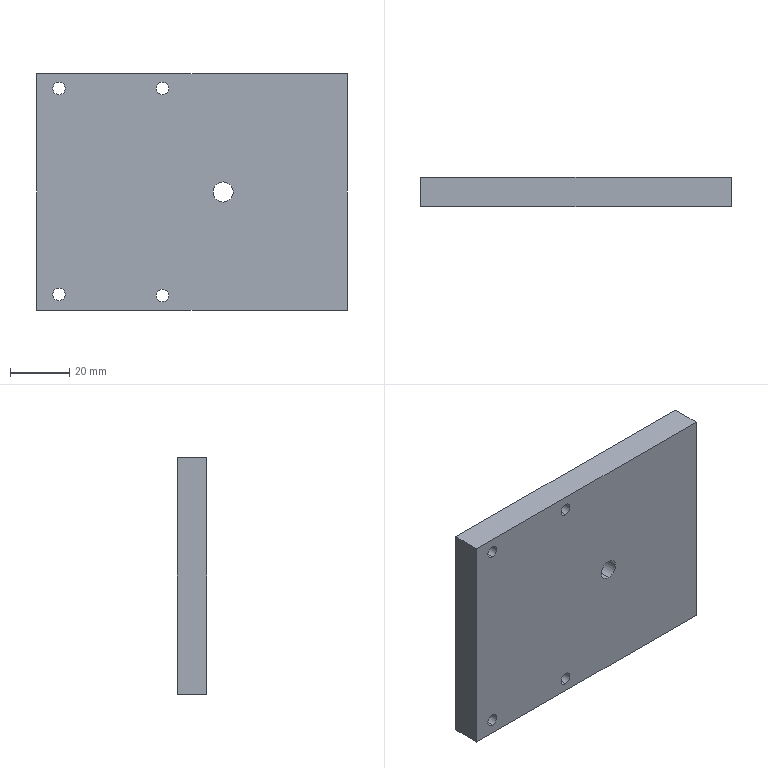Part | STEP file | X77-04021 | 1 solid | 16 faces | box 105 x 10 x 80 mm | volume 83083 mm3 | cylinder 10 | plane 6 | commonest cylinder face diameters 4.2 x8 6.8 x2
STEP:
#1=CARTESIAN_POINT('',(10.5,10.,3.4));
#2=VERTEX_POINT('',#1);
#3=CARTESIAN_POINT('',(10.5,10.,-3.4));
#4=VERTEX_POINT('',#3);
#5=CARTESIAN_POINT('',(10.5,10.,0.));
#6=DIRECTION('',(0.,-1.,0.));
#7=DIRECTION('',(0.,0.,-1.));
#8=AXIS2_PLACEMENT_3D('',#5,#6,#7);
#9=CIRCLE('',#8,3.4);
#10=EDGE_CURVE('',#2,#4,#9,.T.);
#11=ORIENTED_EDGE('',*,*,#10,.F.);
#12=CARTESIAN_POINT('',(10.5,0.,3.4));
#13=VERTEX_POINT('',#12);
#14=CARTESIAN_POINT('',(10.5,0.,3.4));
#15=DIRECTION('',(0.,-1.,0.));
#16=VECTOR('',#15,1000.);
#17=LINE('',#14,#16);
#18=EDGE_CURVE('',#2,#13,#17,.T.);
#19=ORIENTED_EDGE('',*,*,#18,.T.);
#20=CARTESIAN_POINT('',(10.5,0.,-3.4));
#21=VERTEX_POINT('',#20);
#22=CARTESIAN_POINT('',(10.5,0.,0.));
#23=DIRECTION('',(0.,-1.,0.));
#24=DIRECTION('',(0.,0.,-1.));
#25=AXIS2_PLACEMENT_3D('',#22,#23,#24);
#26=CIRCLE('',#25,3.4);
#27=EDGE_CURVE('',#13,#21,#26,.T.);
#28=ORIENTED_EDGE('',*,*,#27,.T.);
#29=CARTESIAN_POINT('',(10.5,0.,-3.4));
#30=DIRECTION('',(0.,-1.,0.));
#31=VECTOR('',#30,1000.);
#32=LINE('',#29,#31);
#33=EDGE_CURVE('',#4,#21,#32,.T.);
#34=ORIENTED_EDGE('',*,*,#33,.F.);
#35=EDGE_LOOP('',(#11,#19,#28,#34));
#36=FACE_OUTER_BOUND('',#35,.T.);
#37=CARTESIAN_POINT('',(10.5,0.,0.));
#38=DIRECTION('',(0.,-1.,0.));
#39=DIRECTION('',(0.,0.,-1.));
#40=AXIS2_PLACEMENT_3D('',#37,#38,#39);
#41=CYLINDRICAL_SURFACE('',#40,3.4);
#42=ADVANCED_FACE('',(#36),#41,.F.);
#43=CARTESIAN_POINT('',(-45.,0.,-32.551));
#44=VERTEX_POINT('',#43);
#45=CARTESIAN_POINT('',(-45.,0.,-36.751));
#46=VERTEX_POINT('',#45);
#47=CARTESIAN_POINT('',(-45.,0.,-34.651));
#48=DIRECTION('',(0.,-1.,0.));
#49=DIRECTION('',(0.,0.,-1.));
#50=AXIS2_PLACEMENT_3D('',#47,#48,#49);
#51=CIRCLE('',#50,2.1);
#52=EDGE_CURVE('',#44,#46,#51,.T.);
#53=ORIENTED_EDGE('',*,*,#52,.T.);
#54=CARTESIAN_POINT('',(-45.,10.,-36.751));
#55=VERTEX_POINT('',#54);
#56=CARTESIAN_POINT('',(-45.,10.,-36.751));
#57=DIRECTION('',(0.,1.,0.));
#58=VECTOR('',#57,1000.);
#59=LINE('',#56,#58);
#60=EDGE_CURVE('',#46,#55,#59,.T.);
#61=ORIENTED_EDGE('',*,*,#60,.T.);
#62=CARTESIAN_POINT('',(-45.,10.,-32.551));
#63=VERTEX_POINT('',#62);
#64=CARTESIAN_POINT('',(-45.,10.,-34.651));
#65=DIRECTION('',(0.,1.,0.));
#66=DIRECTION('',(0.,0.,1.));
#67=AXIS2_PLACEMENT_3D('',#64,#65,#66);
#68=CIRCLE('',#67,2.1);
#69=EDGE_CURVE('',#55,#63,#68,.T.);
#70=ORIENTED_EDGE('',*,*,#69,.T.);
#71=CARTESIAN_POINT('',(-45.,10.,-32.551));
#72=DIRECTION('',(0.,1.,0.));
#73=VECTOR('',#72,1000.);
#74=LINE('',#71,#73);
#75=EDGE_CURVE('',#44,#63,#74,.T.);
#76=ORIENTED_EDGE('',*,*,#75,.F.);
#77=EDGE_LOOP('',(#53,#61,#70,#76));
#78=FACE_OUTER_BOUND('',#77,.T.);
#79=CARTESIAN_POINT('',(-45.,10.,-34.651));
#80=DIRECTION('',(0.,1.,0.));
#81=DIRECTION('',(0.,0.,1.));
#82=AXIS2_PLACEMENT_3D('',#79,#80,#81);
#83=CYLINDRICAL_SURFACE('',#82,2.1);
#84=ADVANCED_FACE('',(#78),#83,.F.);
#85=CARTESIAN_POINT('',(-45.,0.,37.1));
#86=VERTEX_POINT('',#85);
#87=CARTESIAN_POINT('',(-45.,0.,32.9));
#88=VERTEX_POINT('',#87);
#89=CARTESIAN_POINT('',(-45.,0.,35.));
#90=DIRECTION('',(0.,-1.,0.));
#91=DIRECTION('',(0.,0.,-1.));
#92=AXIS2_PLACEMENT_3D('',#89,#90,#91);
#93=CIRCLE('',#92,2.1);
#94=EDGE_CURVE('',#86,#88,#93,.T.);
#95=ORIENTED_EDGE('',*,*,#94,.T.);
#96=CARTESIAN_POINT('',(-45.,10.,32.9));
#97=VERTEX_POINT('',#96);
#98=CARTESIAN_POINT('',(-45.,10.,32.9));
#99=DIRECTION('',(0.,1.,0.));
#100=VECTOR('',#99,1000.);
#101=LINE('',#98,#100);
#102=EDGE_CURVE('',#88,#97,#101,.T.);
#103=ORIENTED_EDGE('',*,*,#102,.T.);
#104=CARTESIAN_POINT('',(-45.,10.,37.1));
#105=VERTEX_POINT('',#104);
#106=CARTESIAN_POINT('',(-45.,10.,35.));
#107=DIRECTION('',(0.,1.,0.));
#108=DIRECTION('',(0.,0.,1.));
#109=AXIS2_PLACEMENT_3D('',#106,#107,#108);
#110=CIRCLE('',#109,2.1);
#111=EDGE_CURVE('',#97,#105,#110,.T.);
#112=ORIENTED_EDGE('',*,*,#111,.T.);
#113=CARTESIAN_POINT('',(-45.,10.,37.1));
#114=DIRECTION('',(0.,1.,0.));
#115=VECTOR('',#114,1000.);
#116=LINE('',#113,#115);
#117=EDGE_CURVE('',#86,#105,#116,.T.);
#118=ORIENTED_EDGE('',*,*,#117,.F.);
#119=EDGE_LOOP('',(#95,#103,#112,#118));
#120=FACE_OUTER_BOUND('',#119,.T.);
#121=CARTESIAN_POINT('',(-45.,10.,35.));
#122=DIRECTION('',(0.,1.,0.));
#123=DIRECTION('',(0.,0.,1.));
#124=AXIS2_PLACEMENT_3D('',#121,#122,#123);
#125=CYLINDRICAL_SURFACE('',#124,2.1);
#126=ADVANCED_FACE('',(#120),#125,.F.);
#127=CARTESIAN_POINT('',(-10.,0.,37.1));
#128=VERTEX_POINT('',#127);
#129=CARTESIAN_POINT('',(-10.,0.,32.9));
#130=VERTEX_POINT('',#129);
#131=CARTESIAN_POINT('',(-10.,0.,35.));
#132=DIRECTION('',(0.,-1.,0.));
#133=DIRECTION('',(0.,0.,-1.));
#134=AXIS2_PLACEMENT_3D('',#131,#132,#133);
#135=CIRCLE('',#134,2.1);
#136=EDGE_CURVE('',#128,#130,#135,.T.);
#137=ORIENTED_EDGE('',*,*,#136,.T.);
#138=CARTESIAN_POINT('',(-10.,10.,32.9));
#139=VERTEX_POINT('',#138);
#140=CARTESIAN_POINT('',(-10.,10.,32.9));
#141=DIRECTION('',(0.,1.,0.));
#142=VECTOR('',#141,1000.);
#143=LINE('',#140,#142);
#144=EDGE_CURVE('',#130,#139,#143,.T.);
#145=ORIENTED_EDGE('',*,*,#144,.T.);
#146=CARTESIAN_POINT('',(-10.,10.,37.1));
#147=VERTEX_POINT('',#146);
#148=CARTESIAN_POINT('',(-10.,10.,35.));
#149=DIRECTION('',(0.,1.,0.));
#150=DIRECTION('',(0.,0.,1.));
#151=AXIS2_PLACEMENT_3D('',#148,#149,#150);
#152=CIRCLE('',#151,2.1);
#153=EDGE_CURVE('',#139,#147,#152,.T.);
#154=ORIENTED_EDGE('',*,*,#153,.T.);
#155=CARTESIAN_POINT('',(-10.,10.,37.1));
#156=DIRECTION('',(0.,1.,0.));
#157=VECTOR('',#156,1000.);
#158=LINE('',#155,#157);
#159=EDGE_CURVE('',#128,#147,#158,.T.);
#160=ORIENTED_EDGE('',*,*,#159,.F.);
#161=EDGE_LOOP('',(#137,#145,#154,#160));
#162=FACE_OUTER_BOUND('',#161,.T.);
#163=CARTESIAN_POINT('',(-10.,10.,35.));
#164=DIRECTION('',(0.,1.,0.));
#165=DIRECTION('',(0.,0.,1.));
#166=AXIS2_PLACEMENT_3D('',#163,#164,#165);
#167=CYLINDRICAL_SURFACE('',#166,2.1);
#168=ADVANCED_FACE('',(#162),#167,.F.);
#169=CARTESIAN_POINT('',(-10.,0.,-32.9));
#170=VERTEX_POINT('',#169);
#171=CARTESIAN_POINT('',(-10.,0.,-37.1));
#172=VERTEX_POINT('',#171);
#173=CARTESIAN_POINT('',(-10.,0.,-35.));
#174=DIRECTION('',(0.,-1.,0.));
#175=DIRECTION('',(0.,0.,-1.));
#176=AXIS2_PLACEMENT_3D('',#173,#174,#175);
#177=CIRCLE('',#176,2.1);
#178=EDGE_CURVE('',#170,#172,#177,.T.);
#179=ORIENTED_EDGE('',*,*,#178,.T.);
#180=CARTESIAN_POINT('',(-10.,10.,-37.1));
#181=VERTEX_POINT('',#180);
#182=CARTESIAN_POINT('',(-10.,10.,-37.1));
#183=DIRECTION('',(0.,1.,0.));
#184=VECTOR('',#183,1000.);
#185=LINE('',#182,#184);
#186=EDGE_CURVE('',#172,#181,#185,.T.);
#187=ORIENTED_EDGE('',*,*,#186,.T.);
#188=CARTESIAN_POINT('',(-10.,10.,-32.9));
#189=VERTEX_POINT('',#188);
#190=CARTESIAN_POINT('',(-10.,10.,-35.));
#191=DIRECTION('',(0.,1.,0.));
#192=DIRECTION('',(0.,0.,1.));
#193=AXIS2_PLACEMENT_3D('',#190,#191,#192);
#194=CIRCLE('',#193,2.1);
#195=EDGE_CURVE('',#181,#189,#194,.T.);
#196=ORIENTED_EDGE('',*,*,#195,.T.);
#197=CARTESIAN_POINT('',(-10.,10.,-32.9));
#198=DIRECTION('',(0.,1.,0.));
#199=VECTOR('',#198,1000.);
#200=LINE('',#197,#199);
#201=EDGE_CURVE('',#170,#189,#200,.T.);
#202=ORIENTED_EDGE('',*,*,#201,.F.);
#203=EDGE_LOOP('',(#179,#187,#196,#202));
#204=FACE_OUTER_BOUND('',#203,.T.);
#205=CARTESIAN_POINT('',(-10.,10.,-35.));
#206=DIRECTION('',(0.,1.,0.));
#207=DIRECTION('',(0.,0.,1.));
#208=AXIS2_PLACEMENT_3D('',#205,#206,#207);
#209=CYLINDRICAL_SURFACE('',#208,2.1);
#210=ADVANCED_FACE('',(#204),#209,.F.);
#211=CARTESIAN_POINT('',(52.5,0.,40.));
#212=VERTEX_POINT('',#211);
#213=CARTESIAN_POINT('',(52.5,0.,-40.));
#214=VERTEX_POINT('',#213);
#215=CARTESIAN_POINT('',(52.5,0.,40.));
#216=DIRECTION('',(0.,0.,-1.));
#217=VECTOR('',#216,1000.);
#218=LINE('',#215,#217);
#219=EDGE_CURVE('',#212,#214,#218,.T.);
#220=ORIENTED_EDGE('',*,*,#219,.T.);
#221=CARTESIAN_POINT('',(52.5,10.,-40.));
#222=VERTEX_POINT('',#221);
#223=CARTESIAN_POINT('',(52.5,10.,-40.));
#224=DIRECTION('',(0.,-1.,0.));
#225=VECTOR('',#224,1000.);
#226=LINE('',#223,#225);
#227=EDGE_CURVE('',#222,#214,#226,.T.);
#228=ORIENTED_EDGE('',*,*,#227,.F.);
#229=CARTESIAN_POINT('',(52.5,10.,40.));
#230=VERTEX_POINT('',#229);
#231=CARTESIAN_POINT('',(52.5,10.,40.));
#232=DIRECTION('',(0.,0.,-1.));
#233=VECTOR('',#232,1000.);
#234=LINE('',#231,#233);
#235=EDGE_CURVE('',#230,#222,#234,.T.);
#236=ORIENTED_EDGE('',*,*,#235,.F.);
#237=CARTESIAN_POINT('',(52.5,10.,40.));
#238=DIRECTION('',(0.,-1.,0.));
#239=VECTOR('',#238,1000.);
#240=LINE('',#237,#239);
#241=EDGE_CURVE('',#230,#212,#240,.T.);
#242=ORIENTED_EDGE('',*,*,#241,.T.);
#243=EDGE_LOOP('',(#220,#228,#236,#242));
#244=FACE_OUTER_BOUND('',#243,.T.);
#245=CARTESIAN_POINT('',(52.5,10.,40.));
#246=DIRECTION('',(-1.,0.,0.));
#247=DIRECTION('',(0.,0.,1.));
#248=AXIS2_PLACEMENT_3D('',#245,#246,#247);
#249=PLANE('',#248);
#250=ADVANCED_FACE('',(#244),#249,.F.);
#251=CARTESIAN_POINT('',(-52.5,0.,-40.));
#252=VERTEX_POINT('',#251);
#253=CARTESIAN_POINT('',(-52.5,0.,-40.));
#254=DIRECTION('',(-1.,0.,0.));
#255=VECTOR('',#254,1000.);
#256=LINE('',#253,#255);
#257=EDGE_CURVE('',#214,#252,#256,.T.);
#258=ORIENTED_EDGE('',*,*,#257,.T.);
#259=CARTESIAN_POINT('',(-52.5,10.,-40.));
#260=VERTEX_POINT('',#259);
#261=CARTESIAN_POINT('',(-52.5,10.,-40.));
#262=DIRECTION('',(0.,-1.,0.));
#263=VECTOR('',#262,1000.);
#264=LINE('',#261,#263);
#265=EDGE_CURVE('',#260,#252,#264,.T.);
#266=ORIENTED_EDGE('',*,*,#265,.F.);
#267=CARTESIAN_POINT('',(-52.5,10.,-40.));
#268=DIRECTION('',(-1.,0.,0.));
#269=VECTOR('',#268,1000.);
#270=LINE('',#267,#269);
#271=EDGE_CURVE('',#222,#260,#270,.T.);
#272=ORIENTED_EDGE('',*,*,#271,.F.);
#273=ORIENTED_EDGE('',*,*,#227,.T.);
#274=EDGE_LOOP('',(#258,#266,#272,#273));
#275=FACE_OUTER_BOUND('',#274,.T.);
#276=CARTESIAN_POINT('',(-52.5,10.,-40.));
#277=DIRECTION('',(0.,0.,1.));
#278=DIRECTION('',(1.,0.,0.));
#279=AXIS2_PLACEMENT_3D('',#276,#277,#278);
#280=PLANE('',#279);
#281=ADVANCED_FACE('',(#275),#280,.F.);
#282=CARTESIAN_POINT('',(-52.5,0.,40.));
#283=VERTEX_POINT('',#282);
#284=CARTESIAN_POINT('',(-52.5,0.,40.));
#285=DIRECTION('',(0.,0.,1.));
#286=VECTOR('',#285,1000.);
#287=LINE('',#284,#286);
#288=EDGE_CURVE('',#252,#283,#287,.T.);
#289=ORIENTED_EDGE('',*,*,#288,.T.);
#290=CARTESIAN_POINT('',(-52.5,10.,40.));
#291=VERTEX_POINT('',#290);
#292=CARTESIAN_POINT('',(-52.5,10.,40.));
#293=DIRECTION('',(0.,-1.,0.));
#294=VECTOR('',#293,1000.);
#295=LINE('',#292,#294);
#296=EDGE_CURVE('',#291,#283,#295,.T.);
#297=ORIENTED_EDGE('',*,*,#296,.F.);
#298=CARTESIAN_POINT('',(-52.5,10.,40.));
#299=DIRECTION('',(0.,0.,1.));
#300=VECTOR('',#299,1000.);
#301=LINE('',#298,#300);
#302=EDGE_CURVE('',#260,#291,#301,.T.);
#303=ORIENTED_EDGE('',*,*,#302,.F.);
#304=ORIENTED_EDGE('',*,*,#265,.T.);
#305=EDGE_LOOP('',(#289,#297,#303,#304));
#306=FACE_OUTER_BOUND('',#305,.T.);
#307=CARTESIAN_POINT('',(-52.5,10.,40.));
#308=DIRECTION('',(1.,0.,0.));
#309=DIRECTION('',(0.,0.,-1.));
#310=AXIS2_PLACEMENT_3D('',#307,#308,#309);
#311=PLANE('',#310);
#312=ADVANCED_FACE('',(#306),#311,.F.);
#313=CARTESIAN_POINT('',(-52.5,0.,40.));
#314=DIRECTION('',(1.,0.,0.));
#315=VECTOR('',#314,1000.);
#316=LINE('',#313,#315);
#317=EDGE_CURVE('',#283,#212,#316,.T.);
#318=ORIENTED_EDGE('',*,*,#317,.T.);
#319=ORIENTED_EDGE('',*,*,#241,.F.);
#320=CARTESIAN_POINT('',(-52.5,10.,40.));
#321=DIRECTION('',(1.,0.,0.));
#322=VECTOR('',#321,1000.);
#323=LINE('',#320,#322);
#324=EDGE_CURVE('',#291,#230,#323,.T.);
#325=ORIENTED_EDGE('',*,*,#324,.F.);
#326=ORIENTED_EDGE('',*,*,#296,.T.);
#327=EDGE_LOOP('',(#318,#319,#325,#326));
#328=FACE_OUTER_BOUND('',#327,.T.);
#329=CARTESIAN_POINT('',(-52.5,10.,40.));
#330=DIRECTION('',(0.,0.,-1.));
#331=DIRECTION('',(-1.,0.,0.));
#332=AXIS2_PLACEMENT_3D('',#329,#330,#331);
#333=PLANE('',#332);
#334=ADVANCED_FACE('',(#328),#333,.F.);
#335=CARTESIAN_POINT('',(10.5,10.,0.));
#336=DIRECTION('',(0.,-1.,0.));
#337=DIRECTION('',(0.,0.,-1.));
#338=AXIS2_PLACEMENT_3D('',#335,#336,#337);
#339=CIRCLE('',#338,3.4);
#340=EDGE_CURVE('',#4,#2,#339,.T.);
#341=ORIENTED_EDGE('',*,*,#340,.T.);
#342=ORIENTED_EDGE('',*,*,#10,.T.);
#343=EDGE_LOOP('',(#341,#342));
#344=FACE_BOUND('',#343,.T.);
#345=CARTESIAN_POINT('',(-45.,10.,-34.651));
#346=DIRECTION('',(0.,1.,0.));
#347=DIRECTION('',(0.,0.,1.));
#348=AXIS2_PLACEMENT_3D('',#345,#346,#347);
#349=CIRCLE('',#348,2.1);
#350=EDGE_CURVE('',#63,#55,#349,.T.);
#351=ORIENTED_EDGE('',*,*,#350,.F.);
#352=ORIENTED_EDGE('',*,*,#69,.F.);
#353=EDGE_LOOP('',(#351,#352));
#354=FACE_BOUND('',#353,.T.);
#355=CARTESIAN_POINT('',(-45.,10.,35.));
#356=DIRECTION('',(0.,1.,0.));
#357=DIRECTION('',(0.,0.,1.));
#358=AXIS2_PLACEMENT_3D('',#355,#356,#357);
#359=CIRCLE('',#358,2.1);
#360=EDGE_CURVE('',#105,#97,#359,.T.);
#361=ORIENTED_EDGE('',*,*,#360,.F.);
#362=ORIENTED_EDGE('',*,*,#111,.F.);
#363=EDGE_LOOP('',(#361,#362));
#364=FACE_BOUND('',#363,.T.);
#365=CARTESIAN_POINT('',(-10.,10.,35.));
#366=DIRECTION('',(0.,1.,0.));
#367=DIRECTION('',(0.,0.,1.));
#368=AXIS2_PLACEMENT_3D('',#365,#366,#367);
#369=CIRCLE('',#368,2.1);
#370=EDGE_CURVE('',#147,#139,#369,.T.);
#371=ORIENTED_EDGE('',*,*,#370,.F.);
#372=ORIENTED_EDGE('',*,*,#153,.F.);
#373=EDGE_LOOP('',(#371,#372));
#374=FACE_BOUND('',#373,.T.);
#375=CARTESIAN_POINT('',(-10.,10.,-35.));
#376=DIRECTION('',(0.,1.,0.));
#377=DIRECTION('',(0.,0.,1.));
#378=AXIS2_PLACEMENT_3D('',#375,#376,#377);
#379=CIRCLE('',#378,2.1);
#380=EDGE_CURVE('',#189,#181,#379,.T.);
#381=ORIENTED_EDGE('',*,*,#380,.F.);
#382=ORIENTED_EDGE('',*,*,#195,.F.);
#383=EDGE_LOOP('',(#381,#382));
#384=FACE_BOUND('',#383,.T.);
#385=ORIENTED_EDGE('',*,*,#235,.T.);
#386=ORIENTED_EDGE('',*,*,#271,.T.);
#387=ORIENTED_EDGE('',*,*,#302,.T.);
#388=ORIENTED_EDGE('',*,*,#324,.T.);
#389=EDGE_LOOP('',(#385,#386,#387,#388));
#390=FACE_OUTER_BOUND('',#389,.T.);
#391=CARTESIAN_POINT('',(52.5,10.,-40.));
#392=DIRECTION('',(0.,-1.,0.));
#393=DIRECTION('',(0.,0.,-1.));
#394=AXIS2_PLACEMENT_3D('',#391,#392,#393);
#395=PLANE('',#394);
#396=ADVANCED_FACE('',(#344,#354,#364,#374,#384,#390),#395,.F.);
#397=CARTESIAN_POINT('',(10.5,0.,0.));
#398=DIRECTION('',(0.,-1.,0.));
#399=DIRECTION('',(0.,0.,-1.));
#400=AXIS2_PLACEMENT_3D('',#397,#398,#399);
#401=CIRCLE('',#400,3.4);
#402=EDGE_CURVE('',#21,#13,#401,.T.);
#403=ORIENTED_EDGE('',*,*,#402,.F.);
#404=ORIENTED_EDGE('',*,*,#27,.F.);
#405=EDGE_LOOP('',(#403,#404));
#406=FACE_BOUND('',#405,.T.);
#407=ORIENTED_EDGE('',*,*,#52,.F.);
#408=CARTESIAN_POINT('',(-45.,0.,-34.651));
#409=DIRECTION('',(0.,-1.,0.));
#410=DIRECTION('',(0.,0.,-1.));
#411=AXIS2_PLACEMENT_3D('',#408,#409,#410);
#412=CIRCLE('',#411,2.1);
#413=EDGE_CURVE('',#46,#44,#412,.T.);
#414=ORIENTED_EDGE('',*,*,#413,.F.);
#415=EDGE_LOOP('',(#407,#414));
#416=FACE_BOUND('',#415,.T.);
#417=ORIENTED_EDGE('',*,*,#94,.F.);
#418=CARTESIAN_POINT('',(-45.,0.,35.));
#419=DIRECTION('',(0.,-1.,0.));
#420=DIRECTION('',(0.,0.,-1.));
#421=AXIS2_PLACEMENT_3D('',#418,#419,#420);
#422=CIRCLE('',#421,2.1);
#423=EDGE_CURVE('',#88,#86,#422,.T.);
#424=ORIENTED_EDGE('',*,*,#423,.F.);
#425=EDGE_LOOP('',(#417,#424));
#426=FACE_BOUND('',#425,.T.);
#427=ORIENTED_EDGE('',*,*,#136,.F.);
#428=CARTESIAN_POINT('',(-10.,0.,35.));
#429=DIRECTION('',(0.,-1.,0.));
#430=DIRECTION('',(0.,0.,-1.));
#431=AXIS2_PLACEMENT_3D('',#428,#429,#430);
#432=CIRCLE('',#431,2.1);
#433=EDGE_CURVE('',#130,#128,#432,.T.);
#434=ORIENTED_EDGE('',*,*,#433,.F.);
#435=EDGE_LOOP('',(#427,#434));
#436=FACE_BOUND('',#435,.T.);
#437=ORIENTED_EDGE('',*,*,#178,.F.);
#438=CARTESIAN_POINT('',(-10.,0.,-35.));
#439=DIRECTION('',(0.,-1.,0.));
#440=DIRECTION('',(0.,0.,-1.));
#441=AXIS2_PLACEMENT_3D('',#438,#439,#440);
#442=CIRCLE('',#441,2.1);
#443=EDGE_CURVE('',#172,#170,#442,.T.);
#444=ORIENTED_EDGE('',*,*,#443,.F.);
#445=EDGE_LOOP('',(#437,#444));
#446=FACE_BOUND('',#445,.T.);
#447=ORIENTED_EDGE('',*,*,#219,.F.);
#448=ORIENTED_EDGE('',*,*,#317,.F.);
#449=ORIENTED_EDGE('',*,*,#288,.F.);
#450=ORIENTED_EDGE('',*,*,#257,.F.);
#451=EDGE_LOOP('',(#447,#448,#449,#450));
#452=FACE_OUTER_BOUND('',#451,.T.);
#453=CARTESIAN_POINT('',(52.5,0.,-40.));
#454=DIRECTION('',(0.,-1.,0.));
#455=DIRECTION('',(0.,0.,-1.));
#456=AXIS2_PLACEMENT_3D('',#453,#454,#455);
#457=PLANE('',#456);
#458=ADVANCED_FACE('',(#406,#416,#426,#436,#446,#452),#457,.T.);
#459=ORIENTED_EDGE('',*,*,#186,.F.);
#460=ORIENTED_EDGE('',*,*,#443,.T.);
#461=ORIENTED_EDGE('',*,*,#201,.T.);
#462=ORIENTED_EDGE('',*,*,#380,.T.);
#463=EDGE_LOOP('',(#459,#460,#461,#462));
#464=FACE_OUTER_BOUND('',#463,.T.);
#465=CARTESIAN_POINT('',(-10.,10.,-35.));
#466=DIRECTION('',(0.,1.,0.));
#467=DIRECTION('',(0.,0.,1.));
#468=AXIS2_PLACEMENT_3D('',#465,#466,#467);
#469=CYLINDRICAL_SURFACE('',#468,2.1);
#470=ADVANCED_FACE('',(#464),#469,.F.);
#471=ORIENTED_EDGE('',*,*,#144,.F.);
#472=ORIENTED_EDGE('',*,*,#433,.T.);
#473=ORIENTED_EDGE('',*,*,#159,.T.);
#474=ORIENTED_EDGE('',*,*,#370,.T.);
#475=EDGE_LOOP('',(#471,#472,#473,#474));
#476=FACE_OUTER_BOUND('',#475,.T.);
#477=CARTESIAN_POINT('',(-10.,10.,35.));
#478=DIRECTION('',(0.,1.,0.));
#479=DIRECTION('',(0.,0.,1.));
#480=AXIS2_PLACEMENT_3D('',#477,#478,#479);
#481=CYLINDRICAL_SURFACE('',#480,2.1);
#482=ADVANCED_FACE('',(#476),#481,.F.);
#483=ORIENTED_EDGE('',*,*,#102,.F.);
#484=ORIENTED_EDGE('',*,*,#423,.T.);
#485=ORIENTED_EDGE('',*,*,#117,.T.);
#486=ORIENTED_EDGE('',*,*,#360,.T.);
#487=EDGE_LOOP('',(#483,#484,#485,#486));
#488=FACE_OUTER_BOUND('',#487,.T.);
#489=CARTESIAN_POINT('',(-45.,10.,35.));
#490=DIRECTION('',(0.,1.,0.));
#491=DIRECTION('',(0.,0.,1.));
#492=AXIS2_PLACEMENT_3D('',#489,#490,#491);
#493=CYLINDRICAL_SURFACE('',#492,2.1);
#494=ADVANCED_FACE('',(#488),#493,.F.);
#495=ORIENTED_EDGE('',*,*,#60,.F.);
#496=ORIENTED_EDGE('',*,*,#413,.T.);
#497=ORIENTED_EDGE('',*,*,#75,.T.);
#498=ORIENTED_EDGE('',*,*,#350,.T.);
#499=EDGE_LOOP('',(#495,#496,#497,#498));
#500=FACE_OUTER_BOUND('',#499,.T.);
#501=CARTESIAN_POINT('',(-45.,10.,-34.651));
#502=DIRECTION('',(0.,1.,0.));
#503=DIRECTION('',(0.,0.,1.));
#504=AXIS2_PLACEMENT_3D('',#501,#502,#503);
#505=CYLINDRICAL_SURFACE('',#504,2.1);
#506=ADVANCED_FACE('',(#500),#505,.F.);
#507=ORIENTED_EDGE('',*,*,#18,.F.);
#508=ORIENTED_EDGE('',*,*,#340,.F.);
#509=ORIENTED_EDGE('',*,*,#33,.T.);
#510=ORIENTED_EDGE('',*,*,#402,.T.);
#511=EDGE_LOOP('',(#507,#508,#509,#510));
#512=FACE_OUTER_BOUND('',#511,.T.);
#513=CARTESIAN_POINT('',(10.5,0.,0.));
#514=DIRECTION('',(0.,-1.,0.));
#515=DIRECTION('',(0.,0.,-1.));
#516=AXIS2_PLACEMENT_3D('',#513,#514,#515);
#517=CYLINDRICAL_SURFACE('',#516,3.4);
#518=ADVANCED_FACE('',(#512),#517,.F.);
#519=CLOSED_SHELL('',(#42,#84,#126,#168,#210,#250,#281,#312,#334,#396,#458,#470,#482,#494,#506,#518));
#520=MANIFOLD_SOLID_BREP('',#519);
#521=CARTESIAN_POINT('',(0.,0.,0.));
#522=DIRECTION('',(0.,0.,1.));
#523=DIRECTION('',(1.,0.,0.));
#524=AXIS2_PLACEMENT_3D('',#521,#522,#523);
#525=(LENGTH_UNIT()NAMED_UNIT(*)SI_UNIT(.MILLI.,.METRE.));
#526=UNCERTAINTY_MEASURE_WITH_UNIT(LENGTH_MEASURE(0.00001),#525,'','');
#527=(NAMED_UNIT(*)PLANE_ANGLE_UNIT()SI_UNIT($,.RADIAN.));
#528=(NAMED_UNIT(*)SI_UNIT($,.STERADIAN.)SOLID_ANGLE_UNIT());
#529=(GEOMETRIC_REPRESENTATION_CONTEXT(3)GLOBAL_UNCERTAINTY_ASSIGNED_CONTEXT((#526))GLOBAL_UNIT_ASSIGNED_CONTEXT((#525,#527,#528))REPRESENTATION_CONTEXT('',''));
#530=ADVANCED_BREP_SHAPE_REPRESENTATION('',(#520,#524),#529);